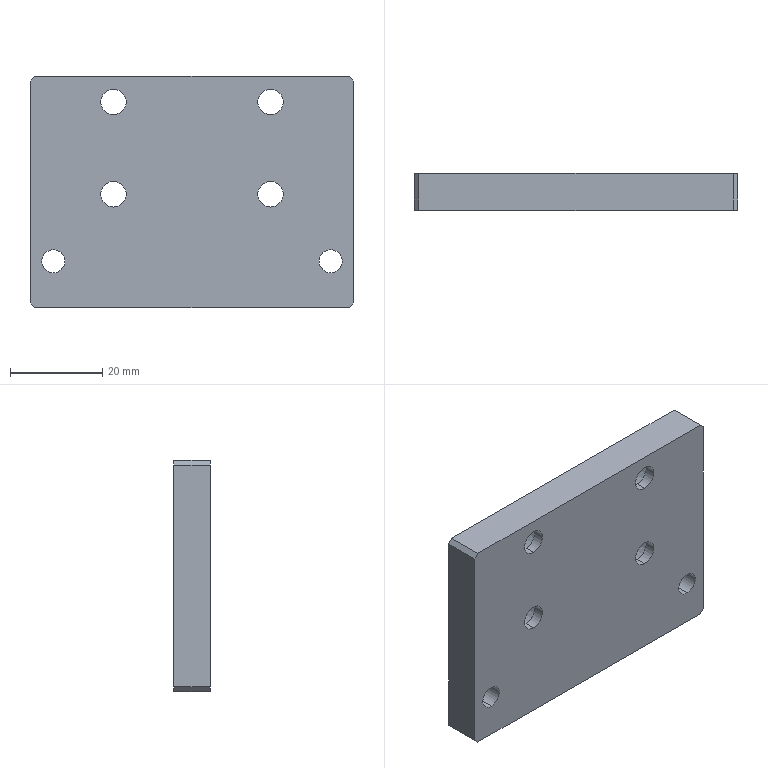Part | STEP file | swing table fixing plate | 1 solid | 34 faces | box 70 x 8 x 50 mm | volume 25661 mm3 | cylinder 20 | plane 14 | commonest cylinder face diameters 5.5 x8 10 x8 5 x4